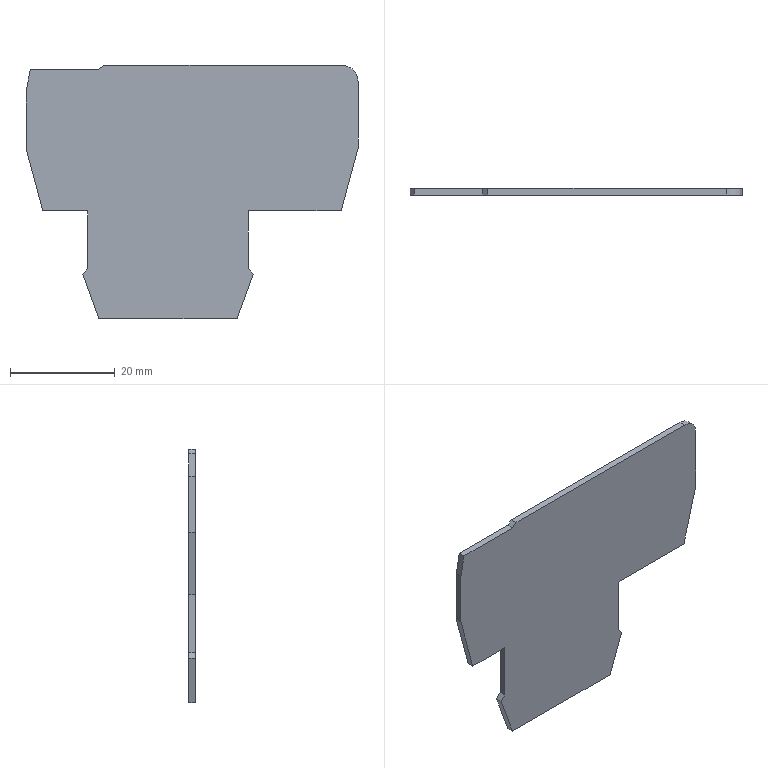Part | SolidWorks | features BaseBody 1 | 1 solid | 21 faces | box 63.246 x 1.25 x 48.204 mm | volume 2895 mm3 | plane 19 | cylinder 2 | commonest cylinder face diameters 1 x1 6 x1
STEP:
#1=CARTESIAN_POINT('',(33.198,-0.625,21.154));
#2=VERTEX_POINT('',#1);
#3=CARTESIAN_POINT('',(36.198,-0.625,18.154));
#4=VERTEX_POINT('',#3);
#5=CARTESIAN_POINT('',(33.198,-0.625,18.154));
#6=DIRECTION('',(0.,1.,0.));
#7=DIRECTION('',(1.,0.,0.));
#8=AXIS2_PLACEMENT_3D('',#5,#6,#7);
#9=CIRCLE('',#8,3.);
#10=EDGE_CURVE('',#2,#4,#9,.T.);
#11=ORIENTED_EDGE('',*,*,#10,.T.);
#12=CARTESIAN_POINT('',(36.198,0.625,18.154));
#13=VERTEX_POINT('',#12);
#14=CARTESIAN_POINT('',(36.198,0.625,18.154));
#15=DIRECTION('',(0.,-1.,0.));
#16=VECTOR('',#15,1000.);
#17=LINE('',#14,#16);
#18=EDGE_CURVE('',#13,#4,#17,.T.);
#19=ORIENTED_EDGE('',*,*,#18,.F.);
#20=CARTESIAN_POINT('',(33.198,0.625,21.154));
#21=VERTEX_POINT('',#20);
#22=CARTESIAN_POINT('',(33.198,0.625,18.154));
#23=DIRECTION('',(0.,1.,0.));
#24=DIRECTION('',(1.,0.,0.));
#25=AXIS2_PLACEMENT_3D('',#22,#23,#24);
#26=CIRCLE('',#25,3.);
#27=EDGE_CURVE('',#21,#13,#26,.T.);
#28=ORIENTED_EDGE('',*,*,#27,.F.);
#29=CARTESIAN_POINT('',(33.198,0.625,21.154));
#30=DIRECTION('',(0.,-1.,0.));
#31=VECTOR('',#30,1000.);
#32=LINE('',#29,#31);
#33=EDGE_CURVE('',#21,#2,#32,.T.);
#34=ORIENTED_EDGE('',*,*,#33,.T.);
#35=EDGE_LOOP('',(#11,#19,#28,#34));
#36=FACE_OUTER_BOUND('',#35,.T.);
#37=CARTESIAN_POINT('',(33.198,0.625,18.154));
#38=DIRECTION('',(0.,-1.,0.));
#39=DIRECTION('',(-1.,0.,0.));
#40=AXIS2_PLACEMENT_3D('',#37,#38,#39);
#41=CYLINDRICAL_SURFACE('',#40,3.);
#42=ADVANCED_FACE('',(#36),#41,.T.);
#43=CARTESIAN_POINT('',(36.198,-0.625,5.409));
#44=VERTEX_POINT('',#43);
#45=CARTESIAN_POINT('',(36.198,-0.625,18.154));
#46=DIRECTION('',(0.,0.,-1.));
#47=VECTOR('',#46,1000.);
#48=LINE('',#45,#47);
#49=EDGE_CURVE('',#4,#44,#48,.T.);
#50=ORIENTED_EDGE('',*,*,#49,.T.);
#51=CARTESIAN_POINT('',(36.198,0.625,5.409));
#52=VERTEX_POINT('',#51);
#53=CARTESIAN_POINT('',(36.198,0.625,5.409));
#54=DIRECTION('',(0.,-1.,0.));
#55=VECTOR('',#54,1000.);
#56=LINE('',#53,#55);
#57=EDGE_CURVE('',#52,#44,#56,.T.);
#58=ORIENTED_EDGE('',*,*,#57,.F.);
#59=CARTESIAN_POINT('',(36.198,0.625,18.154));
#60=DIRECTION('',(0.,0.,-1.));
#61=VECTOR('',#60,1000.);
#62=LINE('',#59,#61);
#63=EDGE_CURVE('',#13,#52,#62,.T.);
#64=ORIENTED_EDGE('',*,*,#63,.F.);
#65=ORIENTED_EDGE('',*,*,#18,.T.);
#66=EDGE_LOOP('',(#50,#58,#64,#65));
#67=FACE_OUTER_BOUND('',#66,.T.);
#68=CARTESIAN_POINT('',(36.198,0.625,18.154));
#69=DIRECTION('',(-1.,0.,0.));
#70=DIRECTION('',(0.,1.,0.));
#71=AXIS2_PLACEMENT_3D('',#68,#69,#70);
#72=PLANE('',#71);
#73=ADVANCED_FACE('',(#67),#72,.F.);
#74=CARTESIAN_POINT('',(33.004,-0.625,-6.512));
#75=VERTEX_POINT('',#74);
#76=CARTESIAN_POINT('',(33.004,-0.625,-6.512));
#77=DIRECTION('',(-0.2588,0.,-0.9659));
#78=VECTOR('',#77,1000.);
#79=LINE('',#76,#78);
#80=EDGE_CURVE('',#44,#75,#79,.T.);
#81=ORIENTED_EDGE('',*,*,#80,.T.);
#82=CARTESIAN_POINT('',(33.004,0.625,-6.512));
#83=VERTEX_POINT('',#82);
#84=CARTESIAN_POINT('',(33.004,0.625,-6.512));
#85=DIRECTION('',(0.,-1.,0.));
#86=VECTOR('',#85,1000.);
#87=LINE('',#84,#86);
#88=EDGE_CURVE('',#83,#75,#87,.T.);
#89=ORIENTED_EDGE('',*,*,#88,.F.);
#90=CARTESIAN_POINT('',(33.004,0.625,-6.512));
#91=DIRECTION('',(-0.2588,0.,-0.9659));
#92=VECTOR('',#91,1000.);
#93=LINE('',#90,#92);
#94=EDGE_CURVE('',#52,#83,#93,.T.);
#95=ORIENTED_EDGE('',*,*,#94,.F.);
#96=ORIENTED_EDGE('',*,*,#57,.T.);
#97=EDGE_LOOP('',(#81,#89,#95,#96));
#98=FACE_OUTER_BOUND('',#97,.T.);
#99=CARTESIAN_POINT('',(33.004,0.625,-6.512));
#100=DIRECTION('',(-0.9659,0.,0.2588));
#101=DIRECTION('',(0.,1.,0.));
#102=AXIS2_PLACEMENT_3D('',#99,#100,#101);
#103=PLANE('',#102);
#104=ADVANCED_FACE('',(#98),#103,.F.);
#105=CARTESIAN_POINT('',(15.313,-0.625,-6.512));
#106=VERTEX_POINT('',#105);
#107=CARTESIAN_POINT('',(33.004,-0.625,-6.512));
#108=DIRECTION('',(-1.,0.,0.));
#109=VECTOR('',#108,1000.);
#110=LINE('',#107,#109);
#111=EDGE_CURVE('',#75,#106,#110,.T.);
#112=ORIENTED_EDGE('',*,*,#111,.T.);
#113=CARTESIAN_POINT('',(15.313,0.625,-6.512));
#114=VERTEX_POINT('',#113);
#115=CARTESIAN_POINT('',(15.313,0.625,-6.512));
#116=DIRECTION('',(0.,-1.,0.));
#117=VECTOR('',#116,1000.);
#118=LINE('',#115,#117);
#119=EDGE_CURVE('',#114,#106,#118,.T.);
#120=ORIENTED_EDGE('',*,*,#119,.F.);
#121=CARTESIAN_POINT('',(33.004,0.625,-6.512));
#122=DIRECTION('',(-1.,0.,0.));
#123=VECTOR('',#122,1000.);
#124=LINE('',#121,#123);
#125=EDGE_CURVE('',#83,#114,#124,.T.);
#126=ORIENTED_EDGE('',*,*,#125,.F.);
#127=ORIENTED_EDGE('',*,*,#88,.T.);
#128=EDGE_LOOP('',(#112,#120,#126,#127));
#129=FACE_OUTER_BOUND('',#128,.T.);
#130=CARTESIAN_POINT('',(33.004,0.625,-6.512));
#131=DIRECTION('',(0.,0.,1.));
#132=DIRECTION('',(1.,0.,0.));
#133=AXIS2_PLACEMENT_3D('',#130,#131,#132);
#134=PLANE('',#133);
#135=ADVANCED_FACE('',(#129),#134,.F.);
#136=CARTESIAN_POINT('',(15.313,-0.625,-17.526));
#137=VERTEX_POINT('',#136);
#138=CARTESIAN_POINT('',(15.313,-0.625,-6.512));
#139=DIRECTION('',(0.,0.,-1.));
#140=VECTOR('',#139,1000.);
#141=LINE('',#138,#140);
#142=EDGE_CURVE('',#106,#137,#141,.T.);
#143=ORIENTED_EDGE('',*,*,#142,.T.);
#144=CARTESIAN_POINT('',(15.313,0.625,-17.526));
#145=VERTEX_POINT('',#144);
#146=CARTESIAN_POINT('',(15.313,0.625,-17.526));
#147=DIRECTION('',(0.,-1.,0.));
#148=VECTOR('',#147,1000.);
#149=LINE('',#146,#148);
#150=EDGE_CURVE('',#145,#137,#149,.T.);
#151=ORIENTED_EDGE('',*,*,#150,.F.);
#152=CARTESIAN_POINT('',(15.313,0.625,-6.512));
#153=DIRECTION('',(0.,0.,-1.));
#154=VECTOR('',#153,1000.);
#155=LINE('',#152,#154);
#156=EDGE_CURVE('',#114,#145,#155,.T.);
#157=ORIENTED_EDGE('',*,*,#156,.F.);
#158=ORIENTED_EDGE('',*,*,#119,.T.);
#159=EDGE_LOOP('',(#143,#151,#157,#158));
#160=FACE_OUTER_BOUND('',#159,.T.);
#161=CARTESIAN_POINT('',(15.313,0.625,-6.512));
#162=DIRECTION('',(-1.,0.,0.));
#163=DIRECTION('',(0.,0.,1.));
#164=AXIS2_PLACEMENT_3D('',#161,#162,#163);
#165=PLANE('',#164);
#166=ADVANCED_FACE('',(#160),#165,.F.);
#167=CARTESIAN_POINT('',(16.221,-0.625,-18.634));
#168=VERTEX_POINT('',#167);
#169=CARTESIAN_POINT('',(15.313,-0.625,-17.526));
#170=DIRECTION('',(0.634,0.,-0.7733));
#171=VECTOR('',#170,1000.);
#172=LINE('',#169,#171);
#173=EDGE_CURVE('',#137,#168,#172,.T.);
#174=ORIENTED_EDGE('',*,*,#173,.T.);
#175=CARTESIAN_POINT('',(16.221,0.625,-18.634));
#176=VERTEX_POINT('',#175);
#177=CARTESIAN_POINT('',(16.221,0.625,-18.634));
#178=DIRECTION('',(0.,-1.,0.));
#179=VECTOR('',#178,1000.);
#180=LINE('',#177,#179);
#181=EDGE_CURVE('',#176,#168,#180,.T.);
#182=ORIENTED_EDGE('',*,*,#181,.F.);
#183=CARTESIAN_POINT('',(15.313,0.625,-17.526));
#184=DIRECTION('',(0.634,0.,-0.7733));
#185=VECTOR('',#184,1000.);
#186=LINE('',#183,#185);
#187=EDGE_CURVE('',#145,#176,#186,.T.);
#188=ORIENTED_EDGE('',*,*,#187,.F.);
#189=ORIENTED_EDGE('',*,*,#150,.T.);
#190=EDGE_LOOP('',(#174,#182,#188,#189));
#191=FACE_OUTER_BOUND('',#190,.T.);
#192=CARTESIAN_POINT('',(15.313,0.625,-17.526));
#193=DIRECTION('',(-0.7733,0.,-0.634));
#194=DIRECTION('',(-0.634,0.,0.7733));
#195=AXIS2_PLACEMENT_3D('',#192,#193,#194);
#196=PLANE('',#195);
#197=ADVANCED_FACE('',(#191),#196,.F.);
#198=CARTESIAN_POINT('',(13.159,-0.625,-27.049));
#199=VERTEX_POINT('',#198);
#200=CARTESIAN_POINT('',(13.159,-0.625,-27.049));
#201=DIRECTION('',(-0.342,0.,-0.9397));
#202=VECTOR('',#201,1000.);
#203=LINE('',#200,#202);
#204=EDGE_CURVE('',#168,#199,#203,.T.);
#205=ORIENTED_EDGE('',*,*,#204,.T.);
#206=CARTESIAN_POINT('',(13.159,0.625,-27.049));
#207=VERTEX_POINT('',#206);
#208=CARTESIAN_POINT('',(13.159,0.625,-27.049));
#209=DIRECTION('',(0.,-1.,0.));
#210=VECTOR('',#209,1000.);
#211=LINE('',#208,#210);
#212=EDGE_CURVE('',#207,#199,#211,.T.);
#213=ORIENTED_EDGE('',*,*,#212,.F.);
#214=CARTESIAN_POINT('',(13.159,0.625,-27.049));
#215=DIRECTION('',(-0.342,0.,-0.9397));
#216=VECTOR('',#215,1000.);
#217=LINE('',#214,#216);
#218=EDGE_CURVE('',#176,#207,#217,.T.);
#219=ORIENTED_EDGE('',*,*,#218,.F.);
#220=ORIENTED_EDGE('',*,*,#181,.T.);
#221=EDGE_LOOP('',(#205,#213,#219,#220));
#222=FACE_OUTER_BOUND('',#221,.T.);
#223=CARTESIAN_POINT('',(13.159,0.625,-27.049));
#224=DIRECTION('',(-0.9397,0.,0.342));
#225=DIRECTION('',(0.,1.,0.));
#226=AXIS2_PLACEMENT_3D('',#223,#224,#225);
#227=PLANE('',#226);
#228=ADVANCED_FACE('',(#222),#227,.F.);
#229=CARTESIAN_POINT('',(-13.159,-0.625,-27.049));
#230=VERTEX_POINT('',#229);
#231=CARTESIAN_POINT('',(-13.159,-0.625,-27.049));
#232=DIRECTION('',(-1.,0.,0.));
#233=VECTOR('',#232,1000.);
#234=LINE('',#231,#233);
#235=EDGE_CURVE('',#199,#230,#234,.T.);
#236=ORIENTED_EDGE('',*,*,#235,.T.);
#237=CARTESIAN_POINT('',(-13.159,0.625,-27.049));
#238=VERTEX_POINT('',#237);
#239=CARTESIAN_POINT('',(-13.159,0.625,-27.049));
#240=DIRECTION('',(0.,-1.,0.));
#241=VECTOR('',#240,1000.);
#242=LINE('',#239,#241);
#243=EDGE_CURVE('',#238,#230,#242,.T.);
#244=ORIENTED_EDGE('',*,*,#243,.F.);
#245=CARTESIAN_POINT('',(-13.159,0.625,-27.049));
#246=DIRECTION('',(-1.,0.,0.));
#247=VECTOR('',#246,1000.);
#248=LINE('',#245,#247);
#249=EDGE_CURVE('',#207,#238,#248,.T.);
#250=ORIENTED_EDGE('',*,*,#249,.F.);
#251=ORIENTED_EDGE('',*,*,#212,.T.);
#252=EDGE_LOOP('',(#236,#244,#250,#251));
#253=FACE_OUTER_BOUND('',#252,.T.);
#254=CARTESIAN_POINT('',(-13.159,0.625,-27.049));
#255=DIRECTION('',(0.,0.,1.));
#256=DIRECTION('',(1.,0.,0.));
#257=AXIS2_PLACEMENT_3D('',#254,#255,#256);
#258=PLANE('',#257);
#259=ADVANCED_FACE('',(#253),#258,.F.);
#260=CARTESIAN_POINT('',(-16.221,-0.625,-18.636));
#261=VERTEX_POINT('',#260);
#262=CARTESIAN_POINT('',(-13.159,-0.625,-27.049));
#263=DIRECTION('',(-0.342,0.,0.9397));
#264=VECTOR('',#263,1000.);
#265=LINE('',#262,#264);
#266=EDGE_CURVE('',#230,#261,#265,.T.);
#267=ORIENTED_EDGE('',*,*,#266,.T.);
#268=CARTESIAN_POINT('',(-16.221,0.625,-18.636));
#269=VERTEX_POINT('',#268);
#270=CARTESIAN_POINT('',(-16.221,0.625,-18.636));
#271=DIRECTION('',(0.,-1.,0.));
#272=VECTOR('',#271,1000.);
#273=LINE('',#270,#272);
#274=EDGE_CURVE('',#269,#261,#273,.T.);
#275=ORIENTED_EDGE('',*,*,#274,.F.);
#276=CARTESIAN_POINT('',(-13.159,0.625,-27.049));
#277=DIRECTION('',(-0.342,0.,0.9397));
#278=VECTOR('',#277,1000.);
#279=LINE('',#276,#278);
#280=EDGE_CURVE('',#238,#269,#279,.T.);
#281=ORIENTED_EDGE('',*,*,#280,.F.);
#282=ORIENTED_EDGE('',*,*,#243,.T.);
#283=EDGE_LOOP('',(#267,#275,#281,#282));
#284=FACE_OUTER_BOUND('',#283,.T.);
#285=CARTESIAN_POINT('',(-13.159,0.625,-27.049));
#286=DIRECTION('',(0.9397,0.,0.342));
#287=DIRECTION('',(0.,-1.,0.));
#288=AXIS2_PLACEMENT_3D('',#285,#286,#287);
#289=PLANE('',#288);
#290=ADVANCED_FACE('',(#284),#289,.F.);
#291=CARTESIAN_POINT('',(-15.262,-0.625,-17.571));
#292=VERTEX_POINT('',#291);
#293=CARTESIAN_POINT('',(-16.221,-0.625,-18.636));
#294=DIRECTION('',(0.6691,0.,0.7431));
#295=VECTOR('',#294,1000.);
#296=LINE('',#293,#295);
#297=EDGE_CURVE('',#261,#292,#296,.T.);
#298=ORIENTED_EDGE('',*,*,#297,.T.);
#299=CARTESIAN_POINT('',(-15.262,0.625,-17.571));
#300=VERTEX_POINT('',#299);
#301=CARTESIAN_POINT('',(-15.262,0.625,-17.571));
#302=DIRECTION('',(0.,-1.,0.));
#303=VECTOR('',#302,1000.);
#304=LINE('',#301,#303);
#305=EDGE_CURVE('',#300,#292,#304,.T.);
#306=ORIENTED_EDGE('',*,*,#305,.F.);
#307=CARTESIAN_POINT('',(-16.221,0.625,-18.636));
#308=DIRECTION('',(0.6691,0.,0.7431));
#309=VECTOR('',#308,1000.);
#310=LINE('',#307,#309);
#311=EDGE_CURVE('',#269,#300,#310,.T.);
#312=ORIENTED_EDGE('',*,*,#311,.F.);
#313=ORIENTED_EDGE('',*,*,#274,.T.);
#314=EDGE_LOOP('',(#298,#306,#312,#313));
#315=FACE_OUTER_BOUND('',#314,.T.);
#316=CARTESIAN_POINT('',(-16.221,0.625,-18.636));
#317=DIRECTION('',(0.7431,0.,-0.6691));
#318=DIRECTION('',(0.,-1.,0.));
#319=AXIS2_PLACEMENT_3D('',#316,#317,#318);
#320=PLANE('',#319);
#321=ADVANCED_FACE('',(#315),#320,.F.);
#322=CARTESIAN_POINT('',(-15.262,-0.625,-6.557));
#323=VERTEX_POINT('',#322);
#324=CARTESIAN_POINT('',(-15.262,-0.625,-17.571));
#325=DIRECTION('',(0.,0.,1.));
#326=VECTOR('',#325,1000.);
#327=LINE('',#324,#326);
#328=EDGE_CURVE('',#292,#323,#327,.T.);
#329=ORIENTED_EDGE('',*,*,#328,.T.);
#330=CARTESIAN_POINT('',(-15.262,0.625,-6.557));
#331=VERTEX_POINT('',#330);
#332=CARTESIAN_POINT('',(-15.262,0.625,-6.557));
#333=DIRECTION('',(0.,-1.,0.));
#334=VECTOR('',#333,1000.);
#335=LINE('',#332,#334);
#336=EDGE_CURVE('',#331,#323,#335,.T.);
#337=ORIENTED_EDGE('',*,*,#336,.F.);
#338=CARTESIAN_POINT('',(-15.262,0.625,-17.571));
#339=DIRECTION('',(0.,0.,1.));
#340=VECTOR('',#339,1000.);
#341=LINE('',#338,#340);
#342=EDGE_CURVE('',#300,#331,#341,.T.);
#343=ORIENTED_EDGE('',*,*,#342,.F.);
#344=ORIENTED_EDGE('',*,*,#305,.T.);
#345=EDGE_LOOP('',(#329,#337,#343,#344));
#346=FACE_OUTER_BOUND('',#345,.T.);
#347=CARTESIAN_POINT('',(-15.262,0.625,-17.571));
#348=DIRECTION('',(1.,0.,0.));
#349=DIRECTION('',(0.,0.,-1.));
#350=AXIS2_PLACEMENT_3D('',#347,#348,#349);
#351=PLANE('',#350);
#352=ADVANCED_FACE('',(#346),#351,.F.);
#353=CARTESIAN_POINT('',(-23.853,-0.625,-6.557));
#354=VERTEX_POINT('',#353);
#355=CARTESIAN_POINT('',(-15.262,-0.625,-6.557));
#356=DIRECTION('',(-1.,0.,0.));
#357=VECTOR('',#356,1000.);
#358=LINE('',#355,#357);
#359=EDGE_CURVE('',#323,#354,#358,.T.);
#360=ORIENTED_EDGE('',*,*,#359,.T.);
#361=CARTESIAN_POINT('',(-23.853,0.625,-6.557));
#362=VERTEX_POINT('',#361);
#363=CARTESIAN_POINT('',(-23.853,0.625,-6.557));
#364=DIRECTION('',(0.,-1.,0.));
#365=VECTOR('',#364,1000.);
#366=LINE('',#363,#365);
#367=EDGE_CURVE('',#362,#354,#366,.T.);
#368=ORIENTED_EDGE('',*,*,#367,.F.);
#369=CARTESIAN_POINT('',(-15.262,0.625,-6.557));
#370=DIRECTION('',(-1.,0.,0.));
#371=VECTOR('',#370,1000.);
#372=LINE('',#369,#371);
#373=EDGE_CURVE('',#331,#362,#372,.T.);
#374=ORIENTED_EDGE('',*,*,#373,.F.);
#375=ORIENTED_EDGE('',*,*,#336,.T.);
#376=EDGE_LOOP('',(#360,#368,#374,#375));
#377=FACE_OUTER_BOUND('',#376,.T.);
#378=CARTESIAN_POINT('',(-15.262,0.625,-6.557));
#379=DIRECTION('',(0.,0.,1.));
#380=DIRECTION('',(1.,0.,0.));
#381=AXIS2_PLACEMENT_3D('',#378,#379,#380);
#382=PLANE('',#381);
#383=ADVANCED_FACE('',(#377),#382,.F.);
#384=CARTESIAN_POINT('',(-27.048,-0.625,5.364));
#385=VERTEX_POINT('',#384);
#386=CARTESIAN_POINT('',(-23.853,-0.625,-6.557));
#387=DIRECTION('',(-0.2588,0.,0.9659));
#388=VECTOR('',#387,1000.);
#389=LINE('',#386,#388);
#390=EDGE_CURVE('',#354,#385,#389,.T.);
#391=ORIENTED_EDGE('',*,*,#390,.T.);
#392=CARTESIAN_POINT('',(-27.048,0.625,5.364));
#393=VERTEX_POINT('',#392);
#394=CARTESIAN_POINT('',(-27.048,0.625,5.364));
#395=DIRECTION('',(0.,-1.,0.));
#396=VECTOR('',#395,1000.);
#397=LINE('',#394,#396);
#398=EDGE_CURVE('',#393,#385,#397,.T.);
#399=ORIENTED_EDGE('',*,*,#398,.F.);
#400=CARTESIAN_POINT('',(-23.853,0.625,-6.557));
#401=DIRECTION('',(-0.2588,0.,0.9659));
#402=VECTOR('',#401,1000.);
#403=LINE('',#400,#402);
#404=EDGE_CURVE('',#362,#393,#403,.T.);
#405=ORIENTED_EDGE('',*,*,#404,.F.);
#406=ORIENTED_EDGE('',*,*,#367,.T.);
#407=EDGE_LOOP('',(#391,#399,#405,#406));
#408=FACE_OUTER_BOUND('',#407,.T.);
#409=CARTESIAN_POINT('',(-23.853,0.625,-6.557));
#410=DIRECTION('',(0.9659,0.,0.2588));
#411=DIRECTION('',(0.,-1.,0.));
#412=AXIS2_PLACEMENT_3D('',#409,#410,#411);
#413=PLANE('',#412);
#414=ADVANCED_FACE('',(#408),#413,.F.);
#415=CARTESIAN_POINT('',(-27.048,-0.625,15.926));
#416=VERTEX_POINT('',#415);
#417=CARTESIAN_POINT('',(-27.048,-0.625,5.364));
#418=DIRECTION('',(0.,0.,1.));
#419=VECTOR('',#418,1000.);
#420=LINE('',#417,#419);
#421=EDGE_CURVE('',#385,#416,#420,.T.);
#422=ORIENTED_EDGE('',*,*,#421,.T.);
#423=CARTESIAN_POINT('',(-27.048,0.625,15.926));
#424=VERTEX_POINT('',#423);
#425=CARTESIAN_POINT('',(-27.048,0.625,15.926));
#426=DIRECTION('',(0.,-1.,0.));
#427=VECTOR('',#426,1000.);
#428=LINE('',#425,#427);
#429=EDGE_CURVE('',#424,#416,#428,.T.);
#430=ORIENTED_EDGE('',*,*,#429,.F.);
#431=CARTESIAN_POINT('',(-27.048,0.625,5.364));
#432=DIRECTION('',(0.,0.,1.));
#433=VECTOR('',#432,1000.);
#434=LINE('',#431,#433);
#435=EDGE_CURVE('',#393,#424,#434,.T.);
#436=ORIENTED_EDGE('',*,*,#435,.F.);
#437=ORIENTED_EDGE('',*,*,#398,.T.);
#438=EDGE_LOOP('',(#422,#430,#436,#437));
#439=FACE_OUTER_BOUND('',#438,.T.);
#440=CARTESIAN_POINT('',(-27.048,0.625,5.364));
#441=DIRECTION('',(1.,0.,0.));
#442=DIRECTION('',(0.,1.,0.));
#443=AXIS2_PLACEMENT_3D('',#440,#441,#442);
#444=PLANE('',#443);
#445=ADVANCED_FACE('',(#439),#444,.F.);
#446=CARTESIAN_POINT('',(-27.039,-0.625,16.016));
#447=VERTEX_POINT('',#446);
#448=CARTESIAN_POINT('',(-26.548,-0.625,15.926));
#449=DIRECTION('',(0.,1.,0.));
#450=DIRECTION('',(1.,0.,0.));
#451=AXIS2_PLACEMENT_3D('',#448,#449,#450);
#452=CIRCLE('',#451,0.5);
#453=EDGE_CURVE('',#416,#447,#452,.T.);
#454=ORIENTED_EDGE('',*,*,#453,.T.);
#455=CARTESIAN_POINT('',(-27.039,0.625,16.016));
#456=VERTEX_POINT('',#455);
#457=CARTESIAN_POINT('',(-27.039,0.625,16.016));
#458=DIRECTION('',(0.,-1.,0.));
#459=VECTOR('',#458,1000.);
#460=LINE('',#457,#459);
#461=EDGE_CURVE('',#456,#447,#460,.T.);
#462=ORIENTED_EDGE('',*,*,#461,.F.);
#463=CARTESIAN_POINT('',(-26.548,0.625,15.926));
#464=DIRECTION('',(0.,1.,0.));
#465=DIRECTION('',(1.,0.,0.));
#466=AXIS2_PLACEMENT_3D('',#463,#464,#465);
#467=CIRCLE('',#466,0.5);
#468=EDGE_CURVE('',#424,#456,#467,.T.);
#469=ORIENTED_EDGE('',*,*,#468,.F.);
#470=ORIENTED_EDGE('',*,*,#429,.T.);
#471=EDGE_LOOP('',(#454,#462,#469,#470));
#472=FACE_OUTER_BOUND('',#471,.T.);
#473=CARTESIAN_POINT('',(-26.548,0.625,15.926));
#474=DIRECTION('',(0.,-1.,0.));
#475=DIRECTION('',(-1.,0.,0.));
#476=AXIS2_PLACEMENT_3D('',#473,#474,#475);
#477=CYLINDRICAL_SURFACE('',#476,0.5);
#478=ADVANCED_FACE('',(#472),#477,.T.);
#479=CARTESIAN_POINT('',(-26.246,-0.625,20.354));
#480=VERTEX_POINT('',#479);
#481=CARTESIAN_POINT('',(-27.039,-0.625,16.016));
#482=DIRECTION('',(0.1799,0.,0.9837));
#483=VECTOR('',#482,1000.);
#484=LINE('',#481,#483);
#485=EDGE_CURVE('',#447,#480,#484,.T.);
#486=ORIENTED_EDGE('',*,*,#485,.T.);
#487=CARTESIAN_POINT('',(-26.246,0.625,20.354));
#488=VERTEX_POINT('',#487);
#489=CARTESIAN_POINT('',(-26.246,0.625,20.354));
#490=DIRECTION('',(0.,-1.,0.));
#491=VECTOR('',#490,1000.);
#492=LINE('',#489,#491);
#493=EDGE_CURVE('',#488,#480,#492,.T.);
#494=ORIENTED_EDGE('',*,*,#493,.F.);
#495=CARTESIAN_POINT('',(-27.039,0.625,16.016));
#496=DIRECTION('',(0.1799,0.,0.9837));
#497=VECTOR('',#496,1000.);
#498=LINE('',#495,#497);
#499=EDGE_CURVE('',#456,#488,#498,.T.);
#500=ORIENTED_EDGE('',*,*,#499,.F.);
#501=ORIENTED_EDGE('',*,*,#461,.T.);
#502=EDGE_LOOP('',(#486,#494,#500,#501));
#503=FACE_OUTER_BOUND('',#502,.T.);
#504=CARTESIAN_POINT('',(-27.039,0.625,16.016));
#505=DIRECTION('',(0.9837,0.,-0.1799));
#506=DIRECTION('',(0.,-1.,0.));
#507=AXIS2_PLACEMENT_3D('',#504,#505,#506);
#508=PLANE('',#507);
#509=ADVANCED_FACE('',(#503),#508,.F.);
#510=CARTESIAN_POINT('',(-13.191,-0.625,20.354));
#511=VERTEX_POINT('',#510);
#512=CARTESIAN_POINT('',(-13.191,-0.625,20.354));
#513=DIRECTION('',(1.,0.,0.));
#514=VECTOR('',#513,1000.);
#515=LINE('',#512,#514);
#516=EDGE_CURVE('',#480,#511,#515,.T.);
#517=ORIENTED_EDGE('',*,*,#516,.T.);
#518=CARTESIAN_POINT('',(-13.191,0.625,20.354));
#519=VERTEX_POINT('',#518);
#520=CARTESIAN_POINT('',(-13.191,0.625,20.354));
#521=DIRECTION('',(0.,-1.,0.));
#522=VECTOR('',#521,1000.);
#523=LINE('',#520,#522);
#524=EDGE_CURVE('',#519,#511,#523,.T.);
#525=ORIENTED_EDGE('',*,*,#524,.F.);
#526=CARTESIAN_POINT('',(-13.191,0.625,20.354));
#527=DIRECTION('',(1.,0.,0.));
#528=VECTOR('',#527,1000.);
#529=LINE('',#526,#528);
#530=EDGE_CURVE('',#488,#519,#529,.T.);
#531=ORIENTED_EDGE('',*,*,#530,.F.);
#532=ORIENTED_EDGE('',*,*,#493,.T.);
#533=EDGE_LOOP('',(#517,#525,#531,#532));
#534=FACE_OUTER_BOUND('',#533,.T.);
#535=CARTESIAN_POINT('',(-13.191,0.625,20.354));
#536=DIRECTION('',(0.,0.,-1.));
#537=DIRECTION('',(-1.,0.,0.));
#538=AXIS2_PLACEMENT_3D('',#535,#536,#537);
#539=PLANE('',#538);
#540=ADVANCED_FACE('',(#534),#539,.F.);
#541=CARTESIAN_POINT('',(-12.216,-0.625,21.154));
#542=VERTEX_POINT('',#541);
#543=CARTESIAN_POINT('',(-12.216,-0.625,21.154));
#544=DIRECTION('',(0.7733,0.,0.634));
#545=VECTOR('',#544,1000.);
#546=LINE('',#543,#545);
#547=EDGE_CURVE('',#511,#542,#546,.T.);
#548=ORIENTED_EDGE('',*,*,#547,.T.);
#549=CARTESIAN_POINT('',(-12.216,0.625,21.154));
#550=VERTEX_POINT('',#549);
#551=CARTESIAN_POINT('',(-12.216,0.625,21.154));
#552=DIRECTION('',(0.,-1.,0.));
#553=VECTOR('',#552,1000.);
#554=LINE('',#551,#553);
#555=EDGE_CURVE('',#550,#542,#554,.T.);
#556=ORIENTED_EDGE('',*,*,#555,.F.);
#557=CARTESIAN_POINT('',(-12.216,0.625,21.154));
#558=DIRECTION('',(0.7733,0.,0.634));
#559=VECTOR('',#558,1000.);
#560=LINE('',#557,#559);
#561=EDGE_CURVE('',#519,#550,#560,.T.);
#562=ORIENTED_EDGE('',*,*,#561,.F.);
#563=ORIENTED_EDGE('',*,*,#524,.T.);
#564=EDGE_LOOP('',(#548,#556,#562,#563));
#565=FACE_OUTER_BOUND('',#564,.T.);
#566=CARTESIAN_POINT('',(-12.216,0.625,21.154));
#567=DIRECTION('',(0.634,0.,-0.7733));
#568=DIRECTION('',(0.,-1.,0.));
#569=AXIS2_PLACEMENT_3D('',#566,#567,#568);
#570=PLANE('',#569);
#571=ADVANCED_FACE('',(#565),#570,.F.);
#572=CARTESIAN_POINT('',(33.198,-0.625,21.154));
#573=DIRECTION('',(1.,0.,0.));
#574=VECTOR('',#573,1000.);
#575=LINE('',#572,#574);
#576=EDGE_CURVE('',#542,#2,#575,.T.);
#577=ORIENTED_EDGE('',*,*,#576,.T.);
#578=ORIENTED_EDGE('',*,*,#33,.F.);
#579=CARTESIAN_POINT('',(33.198,0.625,21.154));
#580=DIRECTION('',(1.,0.,0.));
#581=VECTOR('',#580,1000.);
#582=LINE('',#579,#581);
#583=EDGE_CURVE('',#550,#21,#582,.T.);
#584=ORIENTED_EDGE('',*,*,#583,.F.);
#585=ORIENTED_EDGE('',*,*,#555,.T.);
#586=EDGE_LOOP('',(#577,#578,#584,#585));
#587=FACE_OUTER_BOUND('',#586,.T.);
#588=CARTESIAN_POINT('',(33.198,0.625,21.154));
#589=DIRECTION('',(0.,0.,-1.));
#590=DIRECTION('',(-1.,0.,0.));
#591=AXIS2_PLACEMENT_3D('',#588,#589,#590);
#592=PLANE('',#591);
#593=ADVANCED_FACE('',(#587),#592,.F.);
#594=ORIENTED_EDGE('',*,*,#27,.T.);
#595=ORIENTED_EDGE('',*,*,#63,.T.);
#596=ORIENTED_EDGE('',*,*,#94,.T.);
#597=ORIENTED_EDGE('',*,*,#125,.T.);
#598=ORIENTED_EDGE('',*,*,#156,.T.);
#599=ORIENTED_EDGE('',*,*,#187,.T.);
#600=ORIENTED_EDGE('',*,*,#218,.T.);
#601=ORIENTED_EDGE('',*,*,#249,.T.);
#602=ORIENTED_EDGE('',*,*,#280,.T.);
#603=ORIENTED_EDGE('',*,*,#311,.T.);
#604=ORIENTED_EDGE('',*,*,#342,.T.);
#605=ORIENTED_EDGE('',*,*,#373,.T.);
#606=ORIENTED_EDGE('',*,*,#404,.T.);
#607=ORIENTED_EDGE('',*,*,#435,.T.);
#608=ORIENTED_EDGE('',*,*,#468,.T.);
#609=ORIENTED_EDGE('',*,*,#499,.T.);
#610=ORIENTED_EDGE('',*,*,#530,.T.);
#611=ORIENTED_EDGE('',*,*,#561,.T.);
#612=ORIENTED_EDGE('',*,*,#583,.T.);
#613=EDGE_LOOP('',(#594,#595,#596,#597,#598,#599,#600,#601,#602,#603,#604,#605,#606,#607,#608,#609,#610,#611,#612));
#614=FACE_OUTER_BOUND('',#613,.T.);
#615=CARTESIAN_POINT('',(33.198,0.625,18.154));
#616=DIRECTION('',(0.,1.,0.));
#617=DIRECTION('',(1.,0.,0.));
#618=AXIS2_PLACEMENT_3D('',#615,#616,#617);
#619=PLANE('',#618);
#620=ADVANCED_FACE('',(#614),#619,.T.);
#621=ORIENTED_EDGE('',*,*,#10,.F.);
#622=ORIENTED_EDGE('',*,*,#576,.F.);
#623=ORIENTED_EDGE('',*,*,#547,.F.);
#624=ORIENTED_EDGE('',*,*,#516,.F.);
#625=ORIENTED_EDGE('',*,*,#485,.F.);
#626=ORIENTED_EDGE('',*,*,#453,.F.);
#627=ORIENTED_EDGE('',*,*,#421,.F.);
#628=ORIENTED_EDGE('',*,*,#390,.F.);
#629=ORIENTED_EDGE('',*,*,#359,.F.);
#630=ORIENTED_EDGE('',*,*,#328,.F.);
#631=ORIENTED_EDGE('',*,*,#297,.F.);
#632=ORIENTED_EDGE('',*,*,#266,.F.);
#633=ORIENTED_EDGE('',*,*,#235,.F.);
#634=ORIENTED_EDGE('',*,*,#204,.F.);
#635=ORIENTED_EDGE('',*,*,#173,.F.);
#636=ORIENTED_EDGE('',*,*,#142,.F.);
#637=ORIENTED_EDGE('',*,*,#111,.F.);
#638=ORIENTED_EDGE('',*,*,#80,.F.);
#639=ORIENTED_EDGE('',*,*,#49,.F.);
#640=EDGE_LOOP('',(#621,#622,#623,#624,#625,#626,#627,#628,#629,#630,#631,#632,#633,#634,#635,#636,#637,#638,#639));
#641=FACE_OUTER_BOUND('',#640,.T.);
#642=CARTESIAN_POINT('',(33.198,-0.625,18.154));
#643=DIRECTION('',(0.,1.,0.));
#644=DIRECTION('',(1.,0.,0.));
#645=AXIS2_PLACEMENT_3D('',#642,#643,#644);
#646=PLANE('',#645);
#647=ADVANCED_FACE('',(#641),#646,.F.);
#648=CLOSED_SHELL('',(#42,#73,#104,#135,#166,#197,#228,#259,#290,#321,#352,#383,#414,#445,#478,#509,#540,#571,#593,#620,#647));
#649=MANIFOLD_SOLID_BREP('',#648);
#650=CARTESIAN_POINT('',(0.,0.,0.));
#651=DIRECTION('',(0.,0.,1.));
#652=DIRECTION('',(1.,0.,0.));
#653=AXIS2_PLACEMENT_3D('',#650,#651,#652);
#654=(LENGTH_UNIT()NAMED_UNIT(*)SI_UNIT(.MILLI.,.METRE.));
#655=UNCERTAINTY_MEASURE_WITH_UNIT(LENGTH_MEASURE(0.00001),#654,'','');
#656=(NAMED_UNIT(*)PLANE_ANGLE_UNIT()SI_UNIT($,.RADIAN.));
#657=(NAMED_UNIT(*)SI_UNIT($,.STERADIAN.)SOLID_ANGLE_UNIT());
#658=(GEOMETRIC_REPRESENTATION_CONTEXT(3)GLOBAL_UNCERTAINTY_ASSIGNED_CONTEXT((#655))GLOBAL_UNIT_ASSIGNED_CONTEXT((#654,#656,#657))REPRESENTATION_CONTEXT('',''));
#659=ADVANCED_BREP_SHAPE_REPRESENTATION('',(#649,#653),#658);